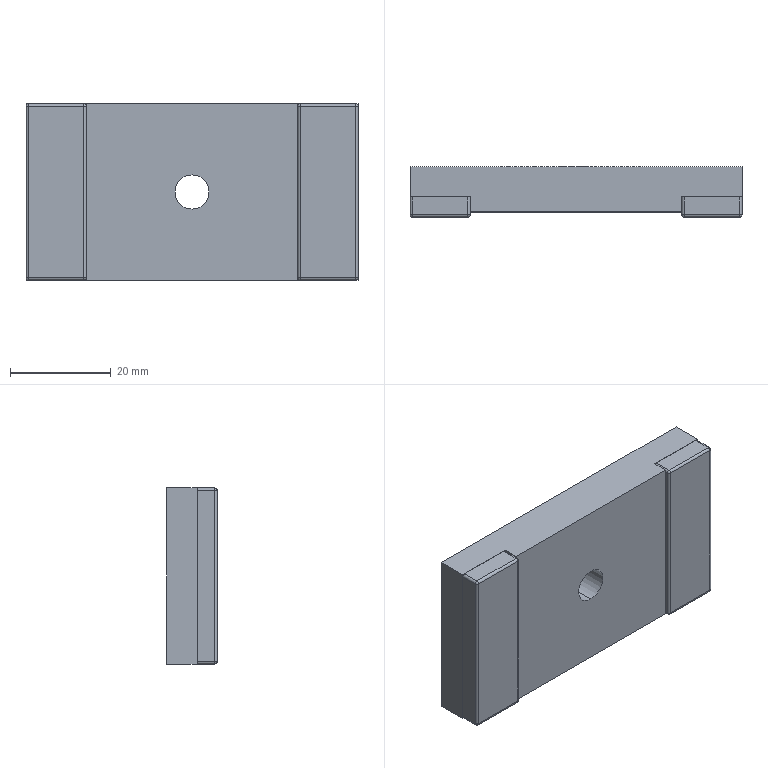Part | SolidWorks | features Fillet 3, Extrusion 1, HoleWzd 1, ICE 1 | 3 solids | 48 faces | box 66 x 10 x 35 mm | volume 21292 mm3 | plane 22 | cylinder 18 | sphere 8 | commonest cylinder face diameters 1 x16 6.8 x2
STEP:
#1=CARTESIAN_POINT('',(-33.,-3.,17.));
#2=VERTEX_POINT('',#1);
#3=CARTESIAN_POINT('',(-33.,-3.,-17.));
#4=VERTEX_POINT('',#3);
#5=CARTESIAN_POINT('',(-33.,-3.,17.5));
#6=DIRECTION('',(0.,0.,-1.));
#7=VECTOR('',#6,1000.);
#8=LINE('',#5,#7);
#9=EDGE_CURVE('',#2,#4,#8,.T.);
#10=ORIENTED_EDGE('',*,*,#9,.T.);
#11=CARTESIAN_POINT('',(-33.,-6.5,-17.));
#12=VERTEX_POINT('',#11);
#13=CARTESIAN_POINT('',(-33.,-7.,-17.));
#14=DIRECTION('',(0.,-1.,0.));
#15=VECTOR('',#14,1000.);
#16=LINE('',#13,#15);
#17=EDGE_CURVE('',#4,#12,#16,.T.);
#18=ORIENTED_EDGE('',*,*,#17,.T.);
#19=CARTESIAN_POINT('',(-33.,-6.5,17.));
#20=VERTEX_POINT('',#19);
#21=CARTESIAN_POINT('',(-33.,-6.5,17.5));
#22=DIRECTION('',(0.,0.,1.));
#23=VECTOR('',#22,1000.);
#24=LINE('',#21,#23);
#25=EDGE_CURVE('',#12,#20,#24,.T.);
#26=ORIENTED_EDGE('',*,*,#25,.T.);
#27=CARTESIAN_POINT('',(-33.,-7.,17.));
#28=DIRECTION('',(0.,1.,0.));
#29=VECTOR('',#28,1000.);
#30=LINE('',#27,#29);
#31=EDGE_CURVE('',#20,#2,#30,.T.);
#32=ORIENTED_EDGE('',*,*,#31,.T.);
#33=EDGE_LOOP('',(#10,#18,#26,#32));
#34=FACE_OUTER_BOUND('',#33,.T.);
#35=CARTESIAN_POINT('',(-33.,-7.,17.5));
#36=DIRECTION('',(1.,0.,0.));
#37=DIRECTION('',(0.,1.,0.));
#38=AXIS2_PLACEMENT_3D('',#35,#36,#37);
#39=PLANE('',#38);
#40=ADVANCED_FACE('',(#34),#39,.F.);
#41=CARTESIAN_POINT('',(-32.5,-3.,-17.5));
#42=VERTEX_POINT('',#41);
#43=CARTESIAN_POINT('',(-21.5,-3.,-17.5));
#44=VERTEX_POINT('',#43);
#45=CARTESIAN_POINT('',(-33.,-3.,-17.5));
#46=DIRECTION('',(1.,0.,0.));
#47=VECTOR('',#46,1000.);
#48=LINE('',#45,#47);
#49=EDGE_CURVE('',#42,#44,#48,.T.);
#50=ORIENTED_EDGE('',*,*,#49,.T.);
#51=CARTESIAN_POINT('',(-21.5,-6.5,-17.5));
#52=VERTEX_POINT('',#51);
#53=CARTESIAN_POINT('',(-21.5,-7.,-17.5));
#54=DIRECTION('',(0.,-1.,0.));
#55=VECTOR('',#54,1000.);
#56=LINE('',#53,#55);
#57=EDGE_CURVE('',#44,#52,#56,.T.);
#58=ORIENTED_EDGE('',*,*,#57,.T.);
#59=CARTESIAN_POINT('',(-32.5,-6.5,-17.5));
#60=VERTEX_POINT('',#59);
#61=CARTESIAN_POINT('',(-33.,-6.5,-17.5));
#62=DIRECTION('',(-1.,0.,0.));
#63=VECTOR('',#62,1000.);
#64=LINE('',#61,#63);
#65=EDGE_CURVE('',#52,#60,#64,.T.);
#66=ORIENTED_EDGE('',*,*,#65,.T.);
#67=CARTESIAN_POINT('',(-32.5,-7.,-17.5));
#68=DIRECTION('',(0.,1.,0.));
#69=VECTOR('',#68,1000.);
#70=LINE('',#67,#69);
#71=EDGE_CURVE('',#60,#42,#70,.T.);
#72=ORIENTED_EDGE('',*,*,#71,.T.);
#73=EDGE_LOOP('',(#50,#58,#66,#72));
#74=FACE_OUTER_BOUND('',#73,.T.);
#75=CARTESIAN_POINT('',(-33.,-7.,-17.5));
#76=DIRECTION('',(0.,0.,1.));
#77=DIRECTION('',(1.,0.,0.));
#78=AXIS2_PLACEMENT_3D('',#75,#76,#77);
#79=PLANE('',#78);
#80=ADVANCED_FACE('',(#74),#79,.F.);
#81=CARTESIAN_POINT('',(-21.,-6.5,17.));
#82=VERTEX_POINT('',#81);
#83=CARTESIAN_POINT('',(-21.,-6.5,-17.));
#84=VERTEX_POINT('',#83);
#85=CARTESIAN_POINT('',(-21.,-6.5,-17.5));
#86=DIRECTION('',(0.,0.,-1.));
#87=VECTOR('',#86,1000.);
#88=LINE('',#85,#87);
#89=EDGE_CURVE('',#82,#84,#88,.T.);
#90=ORIENTED_EDGE('',*,*,#89,.T.);
#91=CARTESIAN_POINT('',(-21.,-3.,-17.));
#92=VERTEX_POINT('',#91);
#93=CARTESIAN_POINT('',(-21.,-7.,-17.));
#94=DIRECTION('',(0.,1.,0.));
#95=VECTOR('',#94,1000.);
#96=LINE('',#93,#95);
#97=EDGE_CURVE('',#84,#92,#96,.T.);
#98=ORIENTED_EDGE('',*,*,#97,.T.);
#99=CARTESIAN_POINT('',(-21.,-3.,17.));
#100=VERTEX_POINT('',#99);
#101=CARTESIAN_POINT('',(-21.,-3.,17.5));
#102=DIRECTION('',(0.,0.,1.));
#103=VECTOR('',#102,1000.);
#104=LINE('',#101,#103);
#105=EDGE_CURVE('',#92,#100,#104,.T.);
#106=ORIENTED_EDGE('',*,*,#105,.T.);
#107=CARTESIAN_POINT('',(-21.,-7.,17.));
#108=DIRECTION('',(0.,-1.,0.));
#109=VECTOR('',#108,1000.);
#110=LINE('',#107,#109);
#111=EDGE_CURVE('',#100,#82,#110,.T.);
#112=ORIENTED_EDGE('',*,*,#111,.T.);
#113=EDGE_LOOP('',(#90,#98,#106,#112));
#114=FACE_OUTER_BOUND('',#113,.T.);
#115=CARTESIAN_POINT('',(-21.,-7.,17.5));
#116=DIRECTION('',(-1.,0.,0.));
#117=DIRECTION('',(0.,-1.,0.));
#118=AXIS2_PLACEMENT_3D('',#115,#116,#117);
#119=PLANE('',#118);
#120=ADVANCED_FACE('',(#114),#119,.F.);
#121=CARTESIAN_POINT('',(-32.5,-6.5,17.5));
#122=VERTEX_POINT('',#121);
#123=CARTESIAN_POINT('',(-21.5,-6.5,17.5));
#124=VERTEX_POINT('',#123);
#125=CARTESIAN_POINT('',(-21.,-6.5,17.5));
#126=DIRECTION('',(1.,0.,0.));
#127=VECTOR('',#126,1000.);
#128=LINE('',#125,#127);
#129=EDGE_CURVE('',#122,#124,#128,.T.);
#130=ORIENTED_EDGE('',*,*,#129,.T.);
#131=CARTESIAN_POINT('',(-21.5,-3.,17.5));
#132=VERTEX_POINT('',#131);
#133=CARTESIAN_POINT('',(-21.5,-7.,17.5));
#134=DIRECTION('',(0.,1.,0.));
#135=VECTOR('',#134,1000.);
#136=LINE('',#133,#135);
#137=EDGE_CURVE('',#124,#132,#136,.T.);
#138=ORIENTED_EDGE('',*,*,#137,.T.);
#139=CARTESIAN_POINT('',(-32.5,-3.,17.5));
#140=VERTEX_POINT('',#139);
#141=CARTESIAN_POINT('',(-33.,-3.,17.5));
#142=DIRECTION('',(-1.,0.,0.));
#143=VECTOR('',#142,1000.);
#144=LINE('',#141,#143);
#145=EDGE_CURVE('',#132,#140,#144,.T.);
#146=ORIENTED_EDGE('',*,*,#145,.T.);
#147=CARTESIAN_POINT('',(-32.5,-7.,17.5));
#148=DIRECTION('',(0.,-1.,0.));
#149=VECTOR('',#148,1000.);
#150=LINE('',#147,#149);
#151=EDGE_CURVE('',#140,#122,#150,.T.);
#152=ORIENTED_EDGE('',*,*,#151,.T.);
#153=EDGE_LOOP('',(#130,#138,#146,#152));
#154=FACE_OUTER_BOUND('',#153,.T.);
#155=CARTESIAN_POINT('',(-33.,-7.,17.5));
#156=DIRECTION('',(0.,0.,-1.));
#157=DIRECTION('',(-1.,0.,0.));
#158=AXIS2_PLACEMENT_3D('',#155,#156,#157);
#159=PLANE('',#158);
#160=ADVANCED_FACE('',(#154),#159,.F.);
#161=CARTESIAN_POINT('',(-21.5,-7.,-17.));
#162=VERTEX_POINT('',#161);
#163=CARTESIAN_POINT('',(-21.5,-7.,17.));
#164=VERTEX_POINT('',#163);
#165=CARTESIAN_POINT('',(-21.5,-7.,17.5));
#166=DIRECTION('',(0.,0.,1.));
#167=VECTOR('',#166,1000.);
#168=LINE('',#165,#167);
#169=EDGE_CURVE('',#162,#164,#168,.T.);
#170=ORIENTED_EDGE('',*,*,#169,.T.);
#171=CARTESIAN_POINT('',(-32.5,-7.,17.));
#172=VERTEX_POINT('',#171);
#173=CARTESIAN_POINT('',(-33.,-7.,17.));
#174=DIRECTION('',(-1.,0.,0.));
#175=VECTOR('',#174,1000.);
#176=LINE('',#173,#175);
#177=EDGE_CURVE('',#164,#172,#176,.T.);
#178=ORIENTED_EDGE('',*,*,#177,.T.);
#179=CARTESIAN_POINT('',(-32.5,-7.,-17.));
#180=VERTEX_POINT('',#179);
#181=CARTESIAN_POINT('',(-32.5,-7.,-17.5));
#182=DIRECTION('',(0.,0.,-1.));
#183=VECTOR('',#182,1000.);
#184=LINE('',#181,#183);
#185=EDGE_CURVE('',#172,#180,#184,.T.);
#186=ORIENTED_EDGE('',*,*,#185,.T.);
#187=CARTESIAN_POINT('',(-21.,-7.,-17.));
#188=DIRECTION('',(1.,0.,0.));
#189=VECTOR('',#188,1000.);
#190=LINE('',#187,#189);
#191=EDGE_CURVE('',#180,#162,#190,.T.);
#192=ORIENTED_EDGE('',*,*,#191,.T.);
#193=EDGE_LOOP('',(#170,#178,#186,#192));
#194=FACE_OUTER_BOUND('',#193,.T.);
#195=CARTESIAN_POINT('',(0.,-7.,0.));
#196=DIRECTION('',(0.,-1.,0.));
#197=DIRECTION('',(1.,0.,0.));
#198=AXIS2_PLACEMENT_3D('',#195,#196,#197);
#199=PLANE('',#198);
#200=ADVANCED_FACE('',(#194),#199,.T.);
#201=ORIENTED_EDGE('',*,*,#105,.F.);
#202=CARTESIAN_POINT('',(-21.5,-3.,-17.));
#203=DIRECTION('',(0.,1.,0.));
#204=DIRECTION('',(1.,0.,0.));
#205=AXIS2_PLACEMENT_3D('',#202,#203,#204);
#206=CIRCLE('',#205,0.5);
#207=EDGE_CURVE('',#92,#44,#206,.T.);
#208=ORIENTED_EDGE('',*,*,#207,.T.);
#209=ORIENTED_EDGE('',*,*,#49,.F.);
#210=CARTESIAN_POINT('',(-32.5,-3.,-17.));
#211=DIRECTION('',(0.,1.,0.));
#212=DIRECTION('',(1.,0.,0.));
#213=AXIS2_PLACEMENT_3D('',#210,#211,#212);
#214=CIRCLE('',#213,0.5);
#215=EDGE_CURVE('',#42,#4,#214,.T.);
#216=ORIENTED_EDGE('',*,*,#215,.T.);
#217=ORIENTED_EDGE('',*,*,#9,.F.);
#218=CARTESIAN_POINT('',(-32.5,-3.,17.));
#219=DIRECTION('',(0.,1.,0.));
#220=DIRECTION('',(1.,0.,0.));
#221=AXIS2_PLACEMENT_3D('',#218,#219,#220);
#222=CIRCLE('',#221,0.5);
#223=EDGE_CURVE('',#2,#140,#222,.T.);
#224=ORIENTED_EDGE('',*,*,#223,.T.);
#225=ORIENTED_EDGE('',*,*,#145,.F.);
#226=CARTESIAN_POINT('',(-21.5,-3.,17.));
#227=DIRECTION('',(0.,1.,0.));
#228=DIRECTION('',(1.,0.,0.));
#229=AXIS2_PLACEMENT_3D('',#226,#227,#228);
#230=CIRCLE('',#229,0.5);
#231=EDGE_CURVE('',#132,#100,#230,.T.);
#232=ORIENTED_EDGE('',*,*,#231,.T.);
#233=EDGE_LOOP('',(#201,#208,#209,#216,#217,#224,#225,#232));
#234=FACE_OUTER_BOUND('',#233,.T.);
#235=CARTESIAN_POINT('',(0.,-3.,0.));
#236=DIRECTION('',(0.,-1.,0.));
#237=DIRECTION('',(1.,0.,0.));
#238=AXIS2_PLACEMENT_3D('',#235,#236,#237);
#239=PLANE('',#238);
#240=ADVANCED_FACE('',(#234),#239,.F.);
#241=ORIENTED_EDGE('',*,*,#65,.F.);
#242=CARTESIAN_POINT('',(-21.5,-6.5,-17.));
#243=DIRECTION('',(-1.,0.,0.));
#244=DIRECTION('',(0.,-1.,0.));
#245=AXIS2_PLACEMENT_3D('',#242,#243,#244);
#246=CIRCLE('',#245,0.5);
#247=EDGE_CURVE('',#52,#162,#246,.T.);
#248=ORIENTED_EDGE('',*,*,#247,.T.);
#249=ORIENTED_EDGE('',*,*,#191,.F.);
#250=CARTESIAN_POINT('',(-32.5,-6.5,-17.));
#251=DIRECTION('',(1.,0.,0.));
#252=DIRECTION('',(0.,-1.,0.));
#253=AXIS2_PLACEMENT_3D('',#250,#251,#252);
#254=CIRCLE('',#253,0.5);
#255=EDGE_CURVE('',#180,#60,#254,.T.);
#256=ORIENTED_EDGE('',*,*,#255,.T.);
#257=EDGE_LOOP('',(#241,#248,#249,#256));
#258=FACE_OUTER_BOUND('',#257,.T.);
#259=CARTESIAN_POINT('',(0.,-6.5,-17.));
#260=DIRECTION('',(-1.,0.,0.));
#261=DIRECTION('',(0.,-1.,0.));
#262=AXIS2_PLACEMENT_3D('',#259,#260,#261);
#263=CYLINDRICAL_SURFACE('',#262,0.5);
#264=ADVANCED_FACE('',(#258),#263,.T.);
#265=ORIENTED_EDGE('',*,*,#169,.F.);
#266=CARTESIAN_POINT('',(-21.5,-6.5,-17.));
#267=DIRECTION('',(0.,0.,1.));
#268=DIRECTION('',(-1.,0.,0.));
#269=AXIS2_PLACEMENT_3D('',#266,#267,#268);
#270=CIRCLE('',#269,0.5);
#271=EDGE_CURVE('',#162,#84,#270,.T.);
#272=ORIENTED_EDGE('',*,*,#271,.T.);
#273=ORIENTED_EDGE('',*,*,#89,.F.);
#274=CARTESIAN_POINT('',(-21.5,-6.5,17.));
#275=DIRECTION('',(0.,0.,-1.));
#276=DIRECTION('',(-1.,0.,0.));
#277=AXIS2_PLACEMENT_3D('',#274,#275,#276);
#278=CIRCLE('',#277,0.5);
#279=EDGE_CURVE('',#82,#164,#278,.T.);
#280=ORIENTED_EDGE('',*,*,#279,.T.);
#281=EDGE_LOOP('',(#265,#272,#273,#280));
#282=FACE_OUTER_BOUND('',#281,.T.);
#283=CARTESIAN_POINT('',(-21.5,-6.5,0.));
#284=DIRECTION('',(0.,0.,-1.));
#285=DIRECTION('',(-1.,0.,0.));
#286=AXIS2_PLACEMENT_3D('',#283,#284,#285);
#287=CYLINDRICAL_SURFACE('',#286,0.5);
#288=ADVANCED_FACE('',(#282),#287,.T.);
#289=ORIENTED_EDGE('',*,*,#25,.F.);
#290=CARTESIAN_POINT('',(-32.5,-6.5,-17.));
#291=DIRECTION('',(0.,0.,1.));
#292=DIRECTION('',(1.,0.,0.));
#293=AXIS2_PLACEMENT_3D('',#290,#291,#292);
#294=CIRCLE('',#293,0.5);
#295=EDGE_CURVE('',#12,#180,#294,.T.);
#296=ORIENTED_EDGE('',*,*,#295,.T.);
#297=ORIENTED_EDGE('',*,*,#185,.F.);
#298=CARTESIAN_POINT('',(-32.5,-6.5,17.));
#299=DIRECTION('',(0.,0.,-1.));
#300=DIRECTION('',(1.,0.,0.));
#301=AXIS2_PLACEMENT_3D('',#298,#299,#300);
#302=CIRCLE('',#301,0.5);
#303=EDGE_CURVE('',#172,#20,#302,.T.);
#304=ORIENTED_EDGE('',*,*,#303,.T.);
#305=EDGE_LOOP('',(#289,#296,#297,#304));
#306=FACE_OUTER_BOUND('',#305,.T.);
#307=CARTESIAN_POINT('',(-32.5,-6.5,0.));
#308=DIRECTION('',(0.,0.,1.));
#309=DIRECTION('',(1.,0.,0.));
#310=AXIS2_PLACEMENT_3D('',#307,#308,#309);
#311=CYLINDRICAL_SURFACE('',#310,0.5);
#312=ADVANCED_FACE('',(#306),#311,.T.);
#313=ORIENTED_EDGE('',*,*,#177,.F.);
#314=CARTESIAN_POINT('',(-21.5,-6.5,17.));
#315=DIRECTION('',(-1.,0.,0.));
#316=DIRECTION('',(0.,1.,0.));
#317=AXIS2_PLACEMENT_3D('',#314,#315,#316);
#318=CIRCLE('',#317,0.5);
#319=EDGE_CURVE('',#164,#124,#318,.T.);
#320=ORIENTED_EDGE('',*,*,#319,.T.);
#321=ORIENTED_EDGE('',*,*,#129,.F.);
#322=CARTESIAN_POINT('',(-32.5,-6.5,17.));
#323=DIRECTION('',(1.,0.,0.));
#324=DIRECTION('',(0.,1.,0.));
#325=AXIS2_PLACEMENT_3D('',#322,#323,#324);
#326=CIRCLE('',#325,0.5);
#327=EDGE_CURVE('',#122,#172,#326,.T.);
#328=ORIENTED_EDGE('',*,*,#327,.T.);
#329=EDGE_LOOP('',(#313,#320,#321,#328));
#330=FACE_OUTER_BOUND('',#329,.T.);
#331=CARTESIAN_POINT('',(0.,-6.5,17.));
#332=DIRECTION('',(1.,0.,0.));
#333=DIRECTION('',(0.,1.,0.));
#334=AXIS2_PLACEMENT_3D('',#331,#332,#333);
#335=CYLINDRICAL_SURFACE('',#334,0.5);
#336=ADVANCED_FACE('',(#330),#335,.T.);
#337=ORIENTED_EDGE('',*,*,#207,.F.);
#338=ORIENTED_EDGE('',*,*,#97,.F.);
#339=CARTESIAN_POINT('',(-21.5,-6.5,-17.));
#340=DIRECTION('',(0.,-1.,0.));
#341=DIRECTION('',(1.,0.,0.));
#342=AXIS2_PLACEMENT_3D('',#339,#340,#341);
#343=CIRCLE('',#342,0.5);
#344=EDGE_CURVE('',#52,#84,#343,.T.);
#345=ORIENTED_EDGE('',*,*,#344,.F.);
#346=ORIENTED_EDGE('',*,*,#57,.F.);
#347=EDGE_LOOP('',(#337,#338,#345,#346));
#348=FACE_OUTER_BOUND('',#347,.T.);
#349=CARTESIAN_POINT('',(-21.5,-7.,-17.));
#350=DIRECTION('',(0.,1.,0.));
#351=DIRECTION('',(-1.,0.,0.));
#352=AXIS2_PLACEMENT_3D('',#349,#350,#351);
#353=CYLINDRICAL_SURFACE('',#352,0.5);
#354=ADVANCED_FACE('',(#348),#353,.T.);
#355=ORIENTED_EDGE('',*,*,#271,.F.);
#356=ORIENTED_EDGE('',*,*,#247,.F.);
#357=ORIENTED_EDGE('',*,*,#344,.T.);
#358=EDGE_LOOP('',(#355,#356,#357));
#359=FACE_OUTER_BOUND('',#358,.T.);
#360=CARTESIAN_POINT('',(-21.5,-6.5,-17.));
#361=DIRECTION('',(0.,1.,0.));
#362=DIRECTION('',(1.,0.,0.));
#363=AXIS2_PLACEMENT_3D('',#360,#361,#362);
#364=SPHERICAL_SURFACE('',#363,0.5);
#365=ADVANCED_FACE('',(#359),#364,.T.);
#366=ORIENTED_EDGE('',*,*,#215,.F.);
#367=ORIENTED_EDGE('',*,*,#71,.F.);
#368=CARTESIAN_POINT('',(-32.5,-6.5,-17.));
#369=DIRECTION('',(0.,-1.,0.));
#370=DIRECTION('',(1.,0.,0.));
#371=AXIS2_PLACEMENT_3D('',#368,#369,#370);
#372=CIRCLE('',#371,0.5);
#373=EDGE_CURVE('',#12,#60,#372,.T.);
#374=ORIENTED_EDGE('',*,*,#373,.F.);
#375=ORIENTED_EDGE('',*,*,#17,.F.);
#376=EDGE_LOOP('',(#366,#367,#374,#375));
#377=FACE_OUTER_BOUND('',#376,.T.);
#378=CARTESIAN_POINT('',(-32.5,-7.,-17.));
#379=DIRECTION('',(0.,1.,0.));
#380=DIRECTION('',(-1.,0.,0.));
#381=AXIS2_PLACEMENT_3D('',#378,#379,#380);
#382=CYLINDRICAL_SURFACE('',#381,0.5);
#383=ADVANCED_FACE('',(#377),#382,.T.);
#384=ORIENTED_EDGE('',*,*,#373,.T.);
#385=ORIENTED_EDGE('',*,*,#255,.F.);
#386=ORIENTED_EDGE('',*,*,#295,.F.);
#387=EDGE_LOOP('',(#384,#385,#386));
#388=FACE_OUTER_BOUND('',#387,.T.);
#389=CARTESIAN_POINT('',(-32.5,-6.5,-17.));
#390=DIRECTION('',(0.,1.,0.));
#391=DIRECTION('',(1.,0.,0.));
#392=AXIS2_PLACEMENT_3D('',#389,#390,#391);
#393=SPHERICAL_SURFACE('',#392,0.5);
#394=ADVANCED_FACE('',(#388),#393,.T.);
#395=ORIENTED_EDGE('',*,*,#231,.F.);
#396=ORIENTED_EDGE('',*,*,#137,.F.);
#397=CARTESIAN_POINT('',(-21.5,-6.5,17.));
#398=DIRECTION('',(0.,-1.,0.));
#399=DIRECTION('',(1.,0.,0.));
#400=AXIS2_PLACEMENT_3D('',#397,#398,#399);
#401=CIRCLE('',#400,0.5);
#402=EDGE_CURVE('',#82,#124,#401,.T.);
#403=ORIENTED_EDGE('',*,*,#402,.F.);
#404=ORIENTED_EDGE('',*,*,#111,.F.);
#405=EDGE_LOOP('',(#395,#396,#403,#404));
#406=FACE_OUTER_BOUND('',#405,.T.);
#407=CARTESIAN_POINT('',(-21.5,-7.,17.));
#408=DIRECTION('',(0.,1.,0.));
#409=DIRECTION('',(-1.,0.,0.));
#410=AXIS2_PLACEMENT_3D('',#407,#408,#409);
#411=CYLINDRICAL_SURFACE('',#410,0.5);
#412=ADVANCED_FACE('',(#406),#411,.T.);
#413=ORIENTED_EDGE('',*,*,#319,.F.);
#414=ORIENTED_EDGE('',*,*,#279,.F.);
#415=ORIENTED_EDGE('',*,*,#402,.T.);
#416=EDGE_LOOP('',(#413,#414,#415));
#417=FACE_OUTER_BOUND('',#416,.T.);
#418=CARTESIAN_POINT('',(-21.5,-6.5,17.));
#419=DIRECTION('',(0.,1.,0.));
#420=DIRECTION('',(1.,0.,0.));
#421=AXIS2_PLACEMENT_3D('',#418,#419,#420);
#422=SPHERICAL_SURFACE('',#421,0.5);
#423=ADVANCED_FACE('',(#417),#422,.T.);
#424=ORIENTED_EDGE('',*,*,#223,.F.);
#425=ORIENTED_EDGE('',*,*,#31,.F.);
#426=CARTESIAN_POINT('',(-32.5,-6.5,17.));
#427=DIRECTION('',(0.,-1.,0.));
#428=DIRECTION('',(1.,0.,0.));
#429=AXIS2_PLACEMENT_3D('',#426,#427,#428);
#430=CIRCLE('',#429,0.5);
#431=EDGE_CURVE('',#122,#20,#430,.T.);
#432=ORIENTED_EDGE('',*,*,#431,.F.);
#433=ORIENTED_EDGE('',*,*,#151,.F.);
#434=EDGE_LOOP('',(#424,#425,#432,#433));
#435=FACE_OUTER_BOUND('',#434,.T.);
#436=CARTESIAN_POINT('',(-32.5,-7.,17.));
#437=DIRECTION('',(0.,1.,0.));
#438=DIRECTION('',(-1.,0.,0.));
#439=AXIS2_PLACEMENT_3D('',#436,#437,#438);
#440=CYLINDRICAL_SURFACE('',#439,0.5);
#441=ADVANCED_FACE('',(#435),#440,.T.);
#442=ORIENTED_EDGE('',*,*,#431,.T.);
#443=ORIENTED_EDGE('',*,*,#303,.F.);
#444=ORIENTED_EDGE('',*,*,#327,.F.);
#445=EDGE_LOOP('',(#442,#443,#444));
#446=FACE_OUTER_BOUND('',#445,.T.);
#447=CARTESIAN_POINT('',(-32.5,-6.5,17.));
#448=DIRECTION('',(0.,1.,0.));
#449=DIRECTION('',(1.,0.,0.));
#450=AXIS2_PLACEMENT_3D('',#447,#448,#449);
#451=SPHERICAL_SURFACE('',#450,0.5);
#452=ADVANCED_FACE('',(#446),#451,.T.);
#453=CLOSED_SHELL('',(#40,#80,#120,#160,#200,#240,#264,#288,#312,#336,#354,#365,#383,#394,#412,#423,#441,#452));
#454=MANIFOLD_SOLID_BREP('',#453);
#455=CARTESIAN_POINT('',(21.,-6.5,-17.));
#456=VERTEX_POINT('',#455);
#457=CARTESIAN_POINT('',(21.,-6.5,17.));
#458=VERTEX_POINT('',#457);
#459=CARTESIAN_POINT('',(21.,-6.5,17.5));
#460=DIRECTION('',(0.,0.,1.));
#461=VECTOR('',#460,1000.);
#462=LINE('',#459,#461);
#463=EDGE_CURVE('',#456,#458,#462,.T.);
#464=ORIENTED_EDGE('',*,*,#463,.T.);
#465=CARTESIAN_POINT('',(21.,-3.,17.));
#466=VERTEX_POINT('',#465);
#467=CARTESIAN_POINT('',(21.,-7.,17.));
#468=DIRECTION('',(0.,1.,0.));
#469=VECTOR('',#468,1000.);
#470=LINE('',#467,#469);
#471=EDGE_CURVE('',#458,#466,#470,.T.);
#472=ORIENTED_EDGE('',*,*,#471,.T.);
#473=CARTESIAN_POINT('',(21.,-3.,-17.));
#474=VERTEX_POINT('',#473);
#475=CARTESIAN_POINT('',(21.,-3.,17.5));
#476=DIRECTION('',(0.,0.,-1.));
#477=VECTOR('',#476,1000.);
#478=LINE('',#475,#477);
#479=EDGE_CURVE('',#466,#474,#478,.T.);
#480=ORIENTED_EDGE('',*,*,#479,.T.);
#481=CARTESIAN_POINT('',(21.,-7.,-17.));
#482=DIRECTION('',(0.,-1.,0.));
#483=VECTOR('',#482,1000.);
#484=LINE('',#481,#483);
#485=EDGE_CURVE('',#474,#456,#484,.T.);
#486=ORIENTED_EDGE('',*,*,#485,.T.);
#487=EDGE_LOOP('',(#464,#472,#480,#486));
#488=FACE_OUTER_BOUND('',#487,.T.);
#489=CARTESIAN_POINT('',(21.,-7.,17.5));
#490=DIRECTION('',(1.,0.,0.));
#491=DIRECTION('',(0.,1.,0.));
#492=AXIS2_PLACEMENT_3D('',#489,#490,#491);
#493=PLANE('',#492);
#494=ADVANCED_FACE('',(#488),#493,.F.);
#495=CARTESIAN_POINT('',(21.5,-3.,-17.5));
#496=VERTEX_POINT('',#495);
#497=CARTESIAN_POINT('',(32.5,-3.,-17.5));
#498=VERTEX_POINT('',#497);
#499=CARTESIAN_POINT('',(21.,-3.,-17.5));
#500=DIRECTION('',(1.,0.,0.));
#501=VECTOR('',#500,1000.);
#502=LINE('',#499,#501);
#503=EDGE_CURVE('',#496,#498,#502,.T.);
#504=ORIENTED_EDGE('',*,*,#503,.T.);
#505=CARTESIAN_POINT('',(32.5,-6.5,-17.5));
#506=VERTEX_POINT('',#505);
#507=CARTESIAN_POINT('',(32.5,-7.,-17.5));
#508=DIRECTION('',(0.,-1.,0.));
#509=VECTOR('',#508,1000.);
#510=LINE('',#507,#509);
#511=EDGE_CURVE('',#498,#506,#510,.T.);
#512=ORIENTED_EDGE('',*,*,#511,.T.);
#513=CARTESIAN_POINT('',(21.5,-6.5,-17.5));
#514=VERTEX_POINT('',#513);
#515=CARTESIAN_POINT('',(21.,-6.5,-17.5));
#516=DIRECTION('',(-1.,0.,0.));
#517=VECTOR('',#516,1000.);
#518=LINE('',#515,#517);
#519=EDGE_CURVE('',#506,#514,#518,.T.);
#520=ORIENTED_EDGE('',*,*,#519,.T.);
#521=CARTESIAN_POINT('',(21.5,-7.,-17.5));
#522=DIRECTION('',(0.,1.,0.));
#523=VECTOR('',#522,1000.);
#524=LINE('',#521,#523);
#525=EDGE_CURVE('',#514,#496,#524,.T.);
#526=ORIENTED_EDGE('',*,*,#525,.T.);
#527=EDGE_LOOP('',(#504,#512,#520,#526));
#528=FACE_OUTER_BOUND('',#527,.T.);
#529=CARTESIAN_POINT('',(21.,-7.,-17.5));
#530=DIRECTION('',(0.,0.,1.));
#531=DIRECTION('',(1.,0.,0.));
#532=AXIS2_PLACEMENT_3D('',#529,#530,#531);
#533=PLANE('',#532);
#534=ADVANCED_FACE('',(#528),#533,.F.);
#535=CARTESIAN_POINT('',(33.,-6.5,17.));
#536=VERTEX_POINT('',#535);
#537=CARTESIAN_POINT('',(33.,-6.5,-17.));
#538=VERTEX_POINT('',#537);
#539=CARTESIAN_POINT('',(33.,-6.5,-17.5));
#540=DIRECTION('',(0.,0.,-1.));
#541=VECTOR('',#540,1000.);
#542=LINE('',#539,#541);
#543=EDGE_CURVE('',#536,#538,#542,.T.);
#544=ORIENTED_EDGE('',*,*,#543,.T.);
#545=CARTESIAN_POINT('',(33.,-3.,-17.));
#546=VERTEX_POINT('',#545);
#547=CARTESIAN_POINT('',(33.,-7.,-17.));
#548=DIRECTION('',(0.,1.,0.));
#549=VECTOR('',#548,1000.);
#550=LINE('',#547,#549);
#551=EDGE_CURVE('',#538,#546,#550,.T.);
#552=ORIENTED_EDGE('',*,*,#551,.T.);
#553=CARTESIAN_POINT('',(33.,-3.,17.));
#554=VERTEX_POINT('',#553);
#555=CARTESIAN_POINT('',(33.,-3.,17.5));
#556=DIRECTION('',(0.,0.,1.));
#557=VECTOR('',#556,1000.);
#558=LINE('',#555,#557);
#559=EDGE_CURVE('',#546,#554,#558,.T.);
#560=ORIENTED_EDGE('',*,*,#559,.T.);
#561=CARTESIAN_POINT('',(33.,-7.,17.));
#562=DIRECTION('',(0.,-1.,0.));
#563=VECTOR('',#562,1000.);
#564=LINE('',#561,#563);
#565=EDGE_CURVE('',#554,#536,#564,.T.);
#566=ORIENTED_EDGE('',*,*,#565,.T.);
#567=EDGE_LOOP('',(#544,#552,#560,#566));
#568=FACE_OUTER_BOUND('',#567,.T.);
#569=CARTESIAN_POINT('',(33.,-7.,17.5));
#570=DIRECTION('',(-1.,0.,0.));
#571=DIRECTION('',(0.,-1.,0.));
#572=AXIS2_PLACEMENT_3D('',#569,#570,#571);
#573=PLANE('',#572);
#574=ADVANCED_FACE('',(#568),#573,.F.);
#575=CARTESIAN_POINT('',(32.5,-3.,17.5));
#576=VERTEX_POINT('',#575);
#577=CARTESIAN_POINT('',(21.5,-3.,17.5));
#578=VERTEX_POINT('',#577);
#579=CARTESIAN_POINT('',(21.,-3.,17.5));
#580=DIRECTION('',(-1.,0.,0.));
#581=VECTOR('',#580,1000.);
#582=LINE('',#579,#581);
#583=EDGE_CURVE('',#576,#578,#582,.T.);
#584=ORIENTED_EDGE('',*,*,#583,.T.);
#585=CARTESIAN_POINT('',(21.5,-6.5,17.5));
#586=VERTEX_POINT('',#585);
#587=CARTESIAN_POINT('',(21.5,-7.,17.5));
#588=DIRECTION('',(0.,-1.,0.));
#589=VECTOR('',#588,1000.);
#590=LINE('',#587,#589);
#591=EDGE_CURVE('',#578,#586,#590,.T.);
#592=ORIENTED_EDGE('',*,*,#591,.T.);
#593=CARTESIAN_POINT('',(32.5,-6.5,17.5));
#594=VERTEX_POINT('',#593);
#595=CARTESIAN_POINT('',(33.,-6.5,17.5));
#596=DIRECTION('',(1.,0.,0.));
#597=VECTOR('',#596,1000.);
#598=LINE('',#595,#597);
#599=EDGE_CURVE('',#586,#594,#598,.T.);
#600=ORIENTED_EDGE('',*,*,#599,.T.);
#601=CARTESIAN_POINT('',(32.5,-7.,17.5));
#602=DIRECTION('',(0.,1.,0.));
#603=VECTOR('',#602,1000.);
#604=LINE('',#601,#603);
#605=EDGE_CURVE('',#594,#576,#604,.T.);
#606=ORIENTED_EDGE('',*,*,#605,.T.);
#607=EDGE_LOOP('',(#584,#592,#600,#606));
#608=FACE_OUTER_BOUND('',#607,.T.);
#609=CARTESIAN_POINT('',(21.,-7.,17.5));
#610=DIRECTION('',(0.,0.,-1.));
#611=DIRECTION('',(-1.,0.,0.));
#612=AXIS2_PLACEMENT_3D('',#609,#610,#611);
#613=PLANE('',#612);
#614=ADVANCED_FACE('',(#608),#613,.F.);
#615=CARTESIAN_POINT('',(32.5,-7.,-17.));
#616=VERTEX_POINT('',#615);
#617=CARTESIAN_POINT('',(32.5,-7.,17.));
#618=VERTEX_POINT('',#617);
#619=CARTESIAN_POINT('',(32.5,-7.,17.5));
#620=DIRECTION('',(0.,0.,1.));
#621=VECTOR('',#620,1000.);
#622=LINE('',#619,#621);
#623=EDGE_CURVE('',#616,#618,#622,.T.);
#624=ORIENTED_EDGE('',*,*,#623,.T.);
#625=CARTESIAN_POINT('',(21.5,-7.,17.));
#626=VERTEX_POINT('',#625);
#627=CARTESIAN_POINT('',(21.,-7.,17.));
#628=DIRECTION('',(-1.,0.,0.));
#629=VECTOR('',#628,1000.);
#630=LINE('',#627,#629);
#631=EDGE_CURVE('',#618,#626,#630,.T.);
#632=ORIENTED_EDGE('',*,*,#631,.T.);
#633=CARTESIAN_POINT('',(21.5,-7.,-17.));
#634=VERTEX_POINT('',#633);
#635=CARTESIAN_POINT('',(21.5,-7.,-17.5));
#636=DIRECTION('',(0.,0.,-1.));
#637=VECTOR('',#636,1000.);
#638=LINE('',#635,#637);
#639=EDGE_CURVE('',#626,#634,#638,.T.);
#640=ORIENTED_EDGE('',*,*,#639,.T.);
#641=CARTESIAN_POINT('',(33.,-7.,-17.));
#642=DIRECTION('',(1.,0.,0.));
#643=VECTOR('',#642,1000.);
#644=LINE('',#641,#643);
#645=EDGE_CURVE('',#634,#616,#644,.T.);
#646=ORIENTED_EDGE('',*,*,#645,.T.);
#647=EDGE_LOOP('',(#624,#632,#640,#646));
#648=FACE_OUTER_BOUND('',#647,.T.);
#649=CARTESIAN_POINT('',(0.,-7.,0.));
#650=DIRECTION('',(0.,-1.,0.));
#651=DIRECTION('',(1.,0.,0.));
#652=AXIS2_PLACEMENT_3D('',#649,#650,#651);
#653=PLANE('',#652);
#654=ADVANCED_FACE('',(#648),#653,.T.);
#655=ORIENTED_EDGE('',*,*,#559,.F.);
#656=CARTESIAN_POINT('',(32.5,-3.,-17.));
#657=DIRECTION('',(0.,1.,0.));
#658=DIRECTION('',(1.,0.,0.));
#659=AXIS2_PLACEMENT_3D('',#656,#657,#658);
#660=CIRCLE('',#659,0.5);
#661=EDGE_CURVE('',#546,#498,#660,.T.);
#662=ORIENTED_EDGE('',*,*,#661,.T.);
#663=ORIENTED_EDGE('',*,*,#503,.F.);
#664=CARTESIAN_POINT('',(21.5,-3.,-17.));
#665=DIRECTION('',(0.,1.,0.));
#666=DIRECTION('',(1.,0.,0.));
#667=AXIS2_PLACEMENT_3D('',#664,#665,#666);
#668=CIRCLE('',#667,0.5);
#669=EDGE_CURVE('',#496,#474,#668,.T.);
#670=ORIENTED_EDGE('',*,*,#669,.T.);
#671=ORIENTED_EDGE('',*,*,#479,.F.);
#672=CARTESIAN_POINT('',(21.5,-3.,17.));
#673=DIRECTION('',(0.,1.,0.));
#674=DIRECTION('',(1.,0.,0.));
#675=AXIS2_PLACEMENT_3D('',#672,#673,#674);
#676=CIRCLE('',#675,0.5);
#677=EDGE_CURVE('',#466,#578,#676,.T.);
#678=ORIENTED_EDGE('',*,*,#677,.T.);
#679=ORIENTED_EDGE('',*,*,#583,.F.);
#680=CARTESIAN_POINT('',(32.5,-3.,17.));
#681=DIRECTION('',(0.,1.,0.));
#682=DIRECTION('',(1.,0.,0.));
#683=AXIS2_PLACEMENT_3D('',#680,#681,#682);
#684=CIRCLE('',#683,0.5);
#685=EDGE_CURVE('',#576,#554,#684,.T.);
#686=ORIENTED_EDGE('',*,*,#685,.T.);
#687=EDGE_LOOP('',(#655,#662,#663,#670,#671,#678,#679,#686));
#688=FACE_OUTER_BOUND('',#687,.T.);
#689=CARTESIAN_POINT('',(0.,-3.,0.));
#690=DIRECTION('',(0.,-1.,0.));
#691=DIRECTION('',(1.,0.,0.));
#692=AXIS2_PLACEMENT_3D('',#689,#690,#691);
#693=PLANE('',#692);
#694=ADVANCED_FACE('',(#688),#693,.F.);
#695=ORIENTED_EDGE('',*,*,#661,.F.);
#696=ORIENTED_EDGE('',*,*,#551,.F.);
#697=CARTESIAN_POINT('',(32.5,-6.5,-17.));
#698=DIRECTION('',(0.,-1.,0.));
#699=DIRECTION('',(1.,0.,0.));
#700=AXIS2_PLACEMENT_3D('',#697,#698,#699);
#701=CIRCLE('',#700,0.5);
#702=EDGE_CURVE('',#506,#538,#701,.T.);
#703=ORIENTED_EDGE('',*,*,#702,.F.);
#704=ORIENTED_EDGE('',*,*,#511,.F.);
#705=EDGE_LOOP('',(#695,#696,#703,#704));
#706=FACE_OUTER_BOUND('',#705,.T.);
#707=CARTESIAN_POINT('',(32.5,-7.,-17.));
#708=DIRECTION('',(0.,1.,0.));
#709=DIRECTION('',(-1.,0.,0.));
#710=AXIS2_PLACEMENT_3D('',#707,#708,#709);
#711=CYLINDRICAL_SURFACE('',#710,0.5);
#712=ADVANCED_FACE('',(#706),#711,.T.);
#713=CARTESIAN_POINT('',(21.5,-6.5,-17.));
#714=DIRECTION('',(-1.,0.,0.));
#715=DIRECTION('',(0.,0.,1.));
#716=AXIS2_PLACEMENT_3D('',#713,#714,#715);
#717=CIRCLE('',#716,0.5);
#718=EDGE_CURVE('',#514,#634,#717,.T.);
#719=ORIENTED_EDGE('',*,*,#718,.F.);
#720=ORIENTED_EDGE('',*,*,#519,.F.);
#721=CARTESIAN_POINT('',(32.5,-6.5,-17.));
#722=DIRECTION('',(1.,0.,0.));
#723=DIRECTION('',(0.,0.,-1.));
#724=AXIS2_PLACEMENT_3D('',#721,#722,#723);
#725=CIRCLE('',#724,0.5);
#726=EDGE_CURVE('',#616,#506,#725,.T.);
#727=ORIENTED_EDGE('',*,*,#726,.F.);
#728=ORIENTED_EDGE('',*,*,#645,.F.);
#729=EDGE_LOOP('',(#719,#720,#727,#728));
#730=FACE_OUTER_BOUND('',#729,.T.);
#731=CARTESIAN_POINT('',(0.,-6.5,-17.));
#732=DIRECTION('',(-1.,0.,0.));
#733=DIRECTION('',(0.,-1.,0.));
#734=AXIS2_PLACEMENT_3D('',#731,#732,#733);
#735=CYLINDRICAL_SURFACE('',#734,0.5);
#736=ADVANCED_FACE('',(#730),#735,.T.);
#737=ORIENTED_EDGE('',*,*,#669,.F.);
#738=ORIENTED_EDGE('',*,*,#525,.F.);
#739=CARTESIAN_POINT('',(21.5,-6.5,-17.));
#740=DIRECTION('',(0.,-1.,0.));
#741=DIRECTION('',(1.,0.,0.));
#742=AXIS2_PLACEMENT_3D('',#739,#740,#741);
#743=CIRCLE('',#742,0.5);
#744=EDGE_CURVE('',#456,#514,#743,.T.);
#745=ORIENTED_EDGE('',*,*,#744,.F.);
#746=ORIENTED_EDGE('',*,*,#485,.F.);
#747=EDGE_LOOP('',(#737,#738,#745,#746));
#748=FACE_OUTER_BOUND('',#747,.T.);
#749=CARTESIAN_POINT('',(21.5,-7.,-17.));
#750=DIRECTION('',(0.,1.,0.));
#751=DIRECTION('',(-1.,0.,0.));
#752=AXIS2_PLACEMENT_3D('',#749,#750,#751);
#753=CYLINDRICAL_SURFACE('',#752,0.5);
#754=ADVANCED_FACE('',(#748),#753,.T.);
#755=ORIENTED_EDGE('',*,*,#726,.T.);
#756=ORIENTED_EDGE('',*,*,#702,.T.);
#757=CARTESIAN_POINT('',(32.5,-6.5,-17.));
#758=DIRECTION('',(0.,0.,1.));
#759=DIRECTION('',(-1.,0.,0.));
#760=AXIS2_PLACEMENT_3D('',#757,#758,#759);
#761=CIRCLE('',#760,0.5);
#762=EDGE_CURVE('',#616,#538,#761,.T.);
#763=ORIENTED_EDGE('',*,*,#762,.F.);
#764=EDGE_LOOP('',(#755,#756,#763));
#765=FACE_OUTER_BOUND('',#764,.T.);
#766=CARTESIAN_POINT('',(32.5,-6.5,-17.));
#767=DIRECTION('',(0.,1.,0.));
#768=DIRECTION('',(-1.,0.,0.));
#769=AXIS2_PLACEMENT_3D('',#766,#767,#768);
#770=SPHERICAL_SURFACE('',#769,0.5);
#771=ADVANCED_FACE('',(#765),#770,.T.);
#772=ORIENTED_EDGE('',*,*,#744,.T.);
#773=ORIENTED_EDGE('',*,*,#718,.T.);
#774=CARTESIAN_POINT('',(21.5,-6.5,-17.));
#775=DIRECTION('',(0.,0.,1.));
#776=DIRECTION('',(-1.,0.,0.));
#777=AXIS2_PLACEMENT_3D('',#774,#775,#776);
#778=CIRCLE('',#777,0.5);
#779=EDGE_CURVE('',#456,#634,#778,.T.);
#780=ORIENTED_EDGE('',*,*,#779,.F.);
#781=EDGE_LOOP('',(#772,#773,#780));
#782=FACE_OUTER_BOUND('',#781,.T.);
#783=CARTESIAN_POINT('',(21.5,-6.5,-17.));
#784=DIRECTION('',(0.,1.,0.));
#785=DIRECTION('',(-1.,0.,0.));
#786=AXIS2_PLACEMENT_3D('',#783,#784,#785);
#787=SPHERICAL_SURFACE('',#786,0.5);
#788=ADVANCED_FACE('',(#782),#787,.T.);
#789=ORIENTED_EDGE('',*,*,#685,.F.);
#790=ORIENTED_EDGE('',*,*,#605,.F.);
#791=CARTESIAN_POINT('',(32.5,-6.5,17.));
#792=DIRECTION('',(0.,-1.,0.));
#793=DIRECTION('',(1.,0.,0.));
#794=AXIS2_PLACEMENT_3D('',#791,#792,#793);
#795=CIRCLE('',#794,0.5);
#796=EDGE_CURVE('',#536,#594,#795,.T.);
#797=ORIENTED_EDGE('',*,*,#796,.F.);
#798=ORIENTED_EDGE('',*,*,#565,.F.);
#799=EDGE_LOOP('',(#789,#790,#797,#798));
#800=FACE_OUTER_BOUND('',#799,.T.);
#801=CARTESIAN_POINT('',(32.5,-7.,17.));
#802=DIRECTION('',(0.,1.,0.));
#803=DIRECTION('',(-1.,0.,0.));
#804=AXIS2_PLACEMENT_3D('',#801,#802,#803);
#805=CYLINDRICAL_SURFACE('',#804,0.5);
#806=ADVANCED_FACE('',(#800),#805,.T.);
#807=ORIENTED_EDGE('',*,*,#762,.T.);
#808=ORIENTED_EDGE('',*,*,#543,.F.);
#809=CARTESIAN_POINT('',(32.5,-6.5,17.));
#810=DIRECTION('',(0.,0.,1.));
#811=DIRECTION('',(1.,0.,0.));
#812=AXIS2_PLACEMENT_3D('',#809,#810,#811);
#813=CIRCLE('',#812,0.5);
#814=EDGE_CURVE('',#618,#536,#813,.T.);
#815=ORIENTED_EDGE('',*,*,#814,.F.);
#816=ORIENTED_EDGE('',*,*,#623,.F.);
#817=EDGE_LOOP('',(#807,#808,#815,#816));
#818=FACE_OUTER_BOUND('',#817,.T.);
#819=CARTESIAN_POINT('',(32.5,-6.5,0.));
#820=DIRECTION('',(0.,0.,-1.));
#821=DIRECTION('',(-1.,0.,0.));
#822=AXIS2_PLACEMENT_3D('',#819,#820,#821);
#823=CYLINDRICAL_SURFACE('',#822,0.5);
#824=ADVANCED_FACE('',(#818),#823,.T.);
#825=ORIENTED_EDGE('',*,*,#779,.T.);
#826=ORIENTED_EDGE('',*,*,#639,.F.);
#827=CARTESIAN_POINT('',(21.5,-6.5,17.));
#828=DIRECTION('',(0.,0.,1.));
#829=DIRECTION('',(1.,0.,0.));
#830=AXIS2_PLACEMENT_3D('',#827,#828,#829);
#831=CIRCLE('',#830,0.5);
#832=EDGE_CURVE('',#458,#626,#831,.T.);
#833=ORIENTED_EDGE('',*,*,#832,.F.);
#834=ORIENTED_EDGE('',*,*,#463,.F.);
#835=EDGE_LOOP('',(#825,#826,#833,#834));
#836=FACE_OUTER_BOUND('',#835,.T.);
#837=CARTESIAN_POINT('',(21.5,-6.5,0.));
#838=DIRECTION('',(0.,0.,1.));
#839=DIRECTION('',(1.,0.,0.));
#840=AXIS2_PLACEMENT_3D('',#837,#838,#839);
#841=CYLINDRICAL_SURFACE('',#840,0.5);
#842=ADVANCED_FACE('',(#836),#841,.T.);
#843=ORIENTED_EDGE('',*,*,#677,.F.);
#844=ORIENTED_EDGE('',*,*,#471,.F.);
#845=CARTESIAN_POINT('',(21.5,-6.5,17.));
#846=DIRECTION('',(0.,-1.,0.));
#847=DIRECTION('',(1.,0.,0.));
#848=AXIS2_PLACEMENT_3D('',#845,#846,#847);
#849=CIRCLE('',#848,0.5);
#850=EDGE_CURVE('',#586,#458,#849,.T.);
#851=ORIENTED_EDGE('',*,*,#850,.F.);
#852=ORIENTED_EDGE('',*,*,#591,.F.);
#853=EDGE_LOOP('',(#843,#844,#851,#852));
#854=FACE_OUTER_BOUND('',#853,.T.);
#855=CARTESIAN_POINT('',(21.5,-7.,17.));
#856=DIRECTION('',(0.,1.,0.));
#857=DIRECTION('',(-1.,0.,0.));
#858=AXIS2_PLACEMENT_3D('',#855,#856,#857);
#859=CYLINDRICAL_SURFACE('',#858,0.5);
#860=ADVANCED_FACE('',(#854),#859,.T.);
#861=ORIENTED_EDGE('',*,*,#814,.T.);
#862=ORIENTED_EDGE('',*,*,#796,.T.);
#863=CARTESIAN_POINT('',(32.5,-6.5,17.));
#864=DIRECTION('',(-1.,0.,0.));
#865=DIRECTION('',(0.,0.,-1.));
#866=AXIS2_PLACEMENT_3D('',#863,#864,#865);
#867=CIRCLE('',#866,0.5);
#868=EDGE_CURVE('',#618,#594,#867,.T.);
#869=ORIENTED_EDGE('',*,*,#868,.F.);
#870=EDGE_LOOP('',(#861,#862,#869));
#871=FACE_OUTER_BOUND('',#870,.T.);
#872=CARTESIAN_POINT('',(32.5,-6.5,17.));
#873=DIRECTION('',(0.,0.,1.));
#874=DIRECTION('',(0.,1.,0.));
#875=AXIS2_PLACEMENT_3D('',#872,#873,#874);
#876=SPHERICAL_SURFACE('',#875,0.5);
#877=ADVANCED_FACE('',(#871),#876,.T.);
#878=ORIENTED_EDGE('',*,*,#850,.T.);
#879=ORIENTED_EDGE('',*,*,#832,.T.);
#880=CARTESIAN_POINT('',(21.5,-6.5,17.));
#881=DIRECTION('',(1.,0.,0.));
#882=DIRECTION('',(0.,0.,1.));
#883=AXIS2_PLACEMENT_3D('',#880,#881,#882);
#884=CIRCLE('',#883,0.5);
#885=EDGE_CURVE('',#586,#626,#884,.T.);
#886=ORIENTED_EDGE('',*,*,#885,.F.);
#887=EDGE_LOOP('',(#878,#879,#886));
#888=FACE_OUTER_BOUND('',#887,.T.);
#889=CARTESIAN_POINT('',(21.5,-6.5,17.));
#890=DIRECTION('',(0.,0.,1.));
#891=DIRECTION('',(0.,-1.,0.));
#892=AXIS2_PLACEMENT_3D('',#889,#890,#891);
#893=SPHERICAL_SURFACE('',#892,0.5);
#894=ADVANCED_FACE('',(#888),#893,.T.);
#895=ORIENTED_EDGE('',*,*,#868,.T.);
#896=ORIENTED_EDGE('',*,*,#599,.F.);
#897=ORIENTED_EDGE('',*,*,#885,.T.);
#898=ORIENTED_EDGE('',*,*,#631,.F.);
#899=EDGE_LOOP('',(#895,#896,#897,#898));
#900=FACE_OUTER_BOUND('',#899,.T.);
#901=CARTESIAN_POINT('',(0.,-6.5,17.));
#902=DIRECTION('',(1.,0.,0.));
#903=DIRECTION('',(0.,1.,0.));
#904=AXIS2_PLACEMENT_3D('',#901,#902,#903);
#905=CYLINDRICAL_SURFACE('',#904,0.5);
#906=ADVANCED_FACE('',(#900),#905,.T.);
#907=CLOSED_SHELL('',(#494,#534,#574,#614,#654,#694,#712,#736,#754,#771,#788,#806,#824,#842,#860,#877,#894,#906));
#908=MANIFOLD_SOLID_BREP('',#907);
#909=CARTESIAN_POINT('',(0.,-6.,-3.4));
#910=VERTEX_POINT('',#909);
#911=CARTESIAN_POINT('',(0.,-6.,3.4));
#912=VERTEX_POINT('',#911);
#913=CARTESIAN_POINT('',(0.,-6.,0.));
#914=DIRECTION('',(0.,1.,0.));
#915=DIRECTION('',(-1.,0.,0.));
#916=AXIS2_PLACEMENT_3D('',#913,#914,#915);
#917=CIRCLE('',#916,3.4);
#918=EDGE_CURVE('',#910,#912,#917,.T.);
#919=ORIENTED_EDGE('',*,*,#918,.F.);
#920=CARTESIAN_POINT('',(0.,3.,-3.4));
#921=VERTEX_POINT('',#920);
#922=CARTESIAN_POINT('',(0.,3.,-3.4));
#923=DIRECTION('',(0.,1.,0.));
#924=VECTOR('',#923,1000.);
#925=LINE('',#922,#924);
#926=EDGE_CURVE('',#910,#921,#925,.T.);
#927=ORIENTED_EDGE('',*,*,#926,.T.);
#928=CARTESIAN_POINT('',(0.,3.,3.4));
#929=VERTEX_POINT('',#928);
#930=CARTESIAN_POINT('',(0.,3.,0.));
#931=DIRECTION('',(0.,1.,0.));
#932=DIRECTION('',(0.,0.,1.));
#933=AXIS2_PLACEMENT_3D('',#930,#931,#932);
#934=CIRCLE('',#933,3.4);
#935=EDGE_CURVE('',#921,#929,#934,.T.);
#936=ORIENTED_EDGE('',*,*,#935,.T.);
#937=CARTESIAN_POINT('',(0.,3.,3.4));
#938=DIRECTION('',(0.,1.,0.));
#939=VECTOR('',#938,1000.);
#940=LINE('',#937,#939);
#941=EDGE_CURVE('',#912,#929,#940,.T.);
#942=ORIENTED_EDGE('',*,*,#941,.F.);
#943=EDGE_LOOP('',(#919,#927,#936,#942));
#944=FACE_OUTER_BOUND('',#943,.T.);
#945=CARTESIAN_POINT('',(0.,3.,0.));
#946=DIRECTION('',(0.,1.,0.));
#947=DIRECTION('',(0.,0.,1.));
#948=AXIS2_PLACEMENT_3D('',#945,#946,#947);
#949=CYLINDRICAL_SURFACE('',#948,3.4);
#950=ADVANCED_FACE('',(#944),#949,.F.);
#951=CARTESIAN_POINT('',(33.,-3.,-17.5));
#952=VERTEX_POINT('',#951);
#953=CARTESIAN_POINT('',(33.,3.,-17.5));
#954=VERTEX_POINT('',#953);
#955=CARTESIAN_POINT('',(33.,-3.,-17.5));
#956=DIRECTION('',(0.,1.,0.));
#957=VECTOR('',#956,1000.);
#958=LINE('',#955,#957);
#959=EDGE_CURVE('',#952,#954,#958,.T.);
#960=ORIENTED_EDGE('',*,*,#959,.T.);
#961=CARTESIAN_POINT('',(33.,3.,17.5));
#962=VERTEX_POINT('',#961);
#963=CARTESIAN_POINT('',(33.,3.,17.5));
#964=DIRECTION('',(0.,0.,-1.));
#965=VECTOR('',#964,1000.);
#966=LINE('',#963,#965);
#967=EDGE_CURVE('',#962,#954,#966,.T.);
#968=ORIENTED_EDGE('',*,*,#967,.F.);
#969=CARTESIAN_POINT('',(33.,-3.,17.5));
#970=VERTEX_POINT('',#969);
#971=CARTESIAN_POINT('',(33.,-3.,17.5));
#972=DIRECTION('',(0.,1.,0.));
#973=VECTOR('',#972,1000.);
#974=LINE('',#971,#973);
#975=EDGE_CURVE('',#970,#962,#974,.T.);
#976=ORIENTED_EDGE('',*,*,#975,.F.);
#977=CARTESIAN_POINT('',(33.,-3.,17.5));
#978=DIRECTION('',(0.,0.,-1.));
#979=VECTOR('',#978,1000.);
#980=LINE('',#977,#979);
#981=EDGE_CURVE('',#970,#952,#980,.T.);
#982=ORIENTED_EDGE('',*,*,#981,.T.);
#983=EDGE_LOOP('',(#960,#968,#976,#982));
#984=FACE_OUTER_BOUND('',#983,.T.);
#985=CARTESIAN_POINT('',(33.,-3.,17.5));
#986=DIRECTION('',(-1.,0.,0.));
#987=DIRECTION('',(0.,0.,1.));
#988=AXIS2_PLACEMENT_3D('',#985,#986,#987);
#989=PLANE('',#988);
#990=ADVANCED_FACE('',(#984),#989,.F.);
#991=CARTESIAN_POINT('',(0.,3.,0.));
#992=DIRECTION('',(0.,1.,0.));
#993=DIRECTION('',(0.,0.,1.));
#994=AXIS2_PLACEMENT_3D('',#991,#992,#993);
#995=CIRCLE('',#994,3.4);
#996=EDGE_CURVE('',#929,#921,#995,.T.);
#997=ORIENTED_EDGE('',*,*,#996,.F.);
#998=ORIENTED_EDGE('',*,*,#935,.F.);
#999=EDGE_LOOP('',(#997,#998));
#1000=FACE_BOUND('',#999,.T.);
#1001=CARTESIAN_POINT('',(-33.,3.,-17.5));
#1002=VERTEX_POINT('',#1001);
#1003=CARTESIAN_POINT('',(-33.,3.,-17.5));
#1004=DIRECTION('',(-1.,0.,0.));
#1005=VECTOR('',#1004,1000.);
#1006=LINE('',#1003,#1005);
#1007=EDGE_CURVE('',#954,#1002,#1006,.T.);
#1008=ORIENTED_EDGE('',*,*,#1007,.T.);
#1009=CARTESIAN_POINT('',(-33.,3.,17.5));
#1010=VERTEX_POINT('',#1009);
#1011=CARTESIAN_POINT('',(-33.,3.,17.5));
#1012=DIRECTION('',(0.,0.,-1.));
#1013=VECTOR('',#1012,1000.);
#1014=LINE('',#1011,#1013);
#1015=EDGE_CURVE('',#1010,#1002,#1014,.T.);
#1016=ORIENTED_EDGE('',*,*,#1015,.F.);
#1017=CARTESIAN_POINT('',(-33.,3.,17.5));
#1018=DIRECTION('',(-1.,0.,0.));
#1019=VECTOR('',#1018,1000.);
#1020=LINE('',#1017,#1019);
#1021=EDGE_CURVE('',#962,#1010,#1020,.T.);
#1022=ORIENTED_EDGE('',*,*,#1021,.F.);
#1023=ORIENTED_EDGE('',*,*,#967,.T.);
#1024=EDGE_LOOP('',(#1008,#1016,#1022,#1023));
#1025=FACE_OUTER_BOUND('',#1024,.T.);
#1026=CARTESIAN_POINT('',(-33.,3.,17.5));
#1027=DIRECTION('',(0.,-1.,0.));
#1028=DIRECTION('',(0.,0.,-1.));
#1029=AXIS2_PLACEMENT_3D('',#1026,#1027,#1028);
#1030=PLANE('',#1029);
#1031=ADVANCED_FACE('',(#1000,#1025),#1030,.F.);
#1032=CARTESIAN_POINT('',(-33.,-3.,-17.5));
#1033=VERTEX_POINT('',#1032);
#1034=CARTESIAN_POINT('',(-33.,-3.,-17.5));
#1035=DIRECTION('',(0.,-1.,0.));
#1036=VECTOR('',#1035,1000.);
#1037=LINE('',#1034,#1036);
#1038=EDGE_CURVE('',#1002,#1033,#1037,.T.);
#1039=ORIENTED_EDGE('',*,*,#1038,.T.);
#1040=CARTESIAN_POINT('',(-33.,-3.,17.5));
#1041=VERTEX_POINT('',#1040);
#1042=CARTESIAN_POINT('',(-33.,-3.,17.5));
#1043=DIRECTION('',(0.,0.,-1.));
#1044=VECTOR('',#1043,1000.);
#1045=LINE('',#1042,#1044);
#1046=EDGE_CURVE('',#1041,#1033,#1045,.T.);
#1047=ORIENTED_EDGE('',*,*,#1046,.F.);
#1048=CARTESIAN_POINT('',(-33.,-3.,17.5));
#1049=DIRECTION('',(0.,-1.,0.));
#1050=VECTOR('',#1049,1000.);
#1051=LINE('',#1048,#1050);
#1052=EDGE_CURVE('',#1010,#1041,#1051,.T.);
#1053=ORIENTED_EDGE('',*,*,#1052,.F.);
#1054=ORIENTED_EDGE('',*,*,#1015,.T.);
#1055=EDGE_LOOP('',(#1039,#1047,#1053,#1054));
#1056=FACE_OUTER_BOUND('',#1055,.T.);
#1057=CARTESIAN_POINT('',(-33.,-3.,17.5));
#1058=DIRECTION('',(1.,0.,0.));
#1059=DIRECTION('',(0.,1.,0.));
#1060=AXIS2_PLACEMENT_3D('',#1057,#1058,#1059);
#1061=PLANE('',#1060);
#1062=ADVANCED_FACE('',(#1056),#1061,.F.);
#1063=CARTESIAN_POINT('',(-21.,-3.,-17.5));
#1064=VERTEX_POINT('',#1063);
#1065=CARTESIAN_POINT('',(-33.,-3.,-17.5));
#1066=DIRECTION('',(1.,0.,0.));
#1067=VECTOR('',#1066,1000.);
#1068=LINE('',#1065,#1067);
#1069=EDGE_CURVE('',#1033,#1064,#1068,.T.);
#1070=ORIENTED_EDGE('',*,*,#1069,.T.);
#1071=CARTESIAN_POINT('',(-21.,-3.,17.5));
#1072=VERTEX_POINT('',#1071);
#1073=CARTESIAN_POINT('',(-21.,-3.,17.5));
#1074=DIRECTION('',(0.,0.,-1.));
#1075=VECTOR('',#1074,1000.);
#1076=LINE('',#1073,#1075);
#1077=EDGE_CURVE('',#1072,#1064,#1076,.T.);
#1078=ORIENTED_EDGE('',*,*,#1077,.F.);
#1079=CARTESIAN_POINT('',(-33.,-3.,17.5));
#1080=DIRECTION('',(1.,0.,0.));
#1081=VECTOR('',#1080,1000.);
#1082=LINE('',#1079,#1081);
#1083=EDGE_CURVE('',#1041,#1072,#1082,.T.);
#1084=ORIENTED_EDGE('',*,*,#1083,.F.);
#1085=ORIENTED_EDGE('',*,*,#1046,.T.);
#1086=EDGE_LOOP('',(#1070,#1078,#1084,#1085));
#1087=FACE_OUTER_BOUND('',#1086,.T.);
#1088=CARTESIAN_POINT('',(-33.,-3.,17.5));
#1089=DIRECTION('',(0.,1.,0.));
#1090=DIRECTION('',(-1.,0.,0.));
#1091=AXIS2_PLACEMENT_3D('',#1088,#1089,#1090);
#1092=PLANE('',#1091);
#1093=ADVANCED_FACE('',(#1087),#1092,.F.);
#1094=CARTESIAN_POINT('',(-21.,-6.,-17.5));
#1095=VERTEX_POINT('',#1094);
#1096=CARTESIAN_POINT('',(-21.,-3.,-17.5));
#1097=DIRECTION('',(0.,-1.,0.));
#1098=VECTOR('',#1097,1000.);
#1099=LINE('',#1096,#1098);
#1100=EDGE_CURVE('',#1064,#1095,#1099,.T.);
#1101=ORIENTED_EDGE('',*,*,#1100,.T.);
#1102=CARTESIAN_POINT('',(-21.,-6.,17.5));
#1103=VERTEX_POINT('',#1102);
#1104=CARTESIAN_POINT('',(-21.,-6.,17.5));
#1105=DIRECTION('',(0.,0.,-1.));
#1106=VECTOR('',#1105,1000.);
#1107=LINE('',#1104,#1106);
#1108=EDGE_CURVE('',#1103,#1095,#1107,.T.);
#1109=ORIENTED_EDGE('',*,*,#1108,.F.);
#1110=CARTESIAN_POINT('',(-21.,-3.,17.5));
#1111=DIRECTION('',(0.,-1.,0.));
#1112=VECTOR('',#1111,1000.);
#1113=LINE('',#1110,#1112);
#1114=EDGE_CURVE('',#1072,#1103,#1113,.T.);
#1115=ORIENTED_EDGE('',*,*,#1114,.F.);
#1116=ORIENTED_EDGE('',*,*,#1077,.T.);
#1117=EDGE_LOOP('',(#1101,#1109,#1115,#1116));
#1118=FACE_OUTER_BOUND('',#1117,.T.);
#1119=CARTESIAN_POINT('',(-21.,-3.,17.5));
#1120=DIRECTION('',(1.,0.,0.));
#1121=DIRECTION('',(0.,0.,-1.));
#1122=AXIS2_PLACEMENT_3D('',#1119,#1120,#1121);
#1123=PLANE('',#1122);
#1124=ADVANCED_FACE('',(#1118),#1123,.F.);
#1125=CARTESIAN_POINT('',(0.,-6.,0.));
#1126=DIRECTION('',(0.,1.,0.));
#1127=DIRECTION('',(-1.,0.,0.));
#1128=AXIS2_PLACEMENT_3D('',#1125,#1126,#1127);
#1129=CIRCLE('',#1128,3.4);
#1130=EDGE_CURVE('',#912,#910,#1129,.T.);
#1131=ORIENTED_EDGE('',*,*,#1130,.T.);
#1132=ORIENTED_EDGE('',*,*,#918,.T.);
#1133=EDGE_LOOP('',(#1131,#1132));
#1134=FACE_BOUND('',#1133,.T.);
#1135=CARTESIAN_POINT('',(21.,-6.,-17.5));
#1136=VERTEX_POINT('',#1135);
#1137=CARTESIAN_POINT('',(-21.,-6.,-17.5));
#1138=DIRECTION('',(1.,0.,0.));
#1139=VECTOR('',#1138,1000.);
#1140=LINE('',#1137,#1139);
#1141=EDGE_CURVE('',#1095,#1136,#1140,.T.);
#1142=ORIENTED_EDGE('',*,*,#1141,.T.);
#1143=CARTESIAN_POINT('',(21.,-6.,17.5));
#1144=VERTEX_POINT('',#1143);
#1145=CARTESIAN_POINT('',(21.,-6.,17.5));
#1146=DIRECTION('',(0.,0.,-1.));
#1147=VECTOR('',#1146,1000.);
#1148=LINE('',#1145,#1147);
#1149=EDGE_CURVE('',#1144,#1136,#1148,.T.);
#1150=ORIENTED_EDGE('',*,*,#1149,.F.);
#1151=CARTESIAN_POINT('',(-21.,-6.,17.5));
#1152=DIRECTION('',(1.,0.,0.));
#1153=VECTOR('',#1152,1000.);
#1154=LINE('',#1151,#1153);
#1155=EDGE_CURVE('',#1103,#1144,#1154,.T.);
#1156=ORIENTED_EDGE('',*,*,#1155,.F.);
#1157=ORIENTED_EDGE('',*,*,#1108,.T.);
#1158=EDGE_LOOP('',(#1142,#1150,#1156,#1157));
#1159=FACE_OUTER_BOUND('',#1158,.T.);
#1160=CARTESIAN_POINT('',(-21.,-6.,17.5));
#1161=DIRECTION('',(0.,1.,0.));
#1162=DIRECTION('',(-1.,0.,0.));
#1163=AXIS2_PLACEMENT_3D('',#1160,#1161,#1162);
#1164=PLANE('',#1163);
#1165=ADVANCED_FACE('',(#1134,#1159),#1164,.F.);
#1166=CARTESIAN_POINT('',(21.,-3.,-17.5));
#1167=VERTEX_POINT('',#1166);
#1168=CARTESIAN_POINT('',(21.,-3.,-17.5));
#1169=DIRECTION('',(0.,1.,0.));
#1170=VECTOR('',#1169,1000.);
#1171=LINE('',#1168,#1170);
#1172=EDGE_CURVE('',#1136,#1167,#1171,.T.);
#1173=ORIENTED_EDGE('',*,*,#1172,.T.);
#1174=CARTESIAN_POINT('',(21.,-3.,17.5));
#1175=VERTEX_POINT('',#1174);
#1176=CARTESIAN_POINT('',(21.,-3.,17.5));
#1177=DIRECTION('',(0.,0.,-1.));
#1178=VECTOR('',#1177,1000.);
#1179=LINE('',#1176,#1178);
#1180=EDGE_CURVE('',#1175,#1167,#1179,.T.);
#1181=ORIENTED_EDGE('',*,*,#1180,.F.);
#1182=CARTESIAN_POINT('',(21.,-3.,17.5));
#1183=DIRECTION('',(0.,1.,0.));
#1184=VECTOR('',#1183,1000.);
#1185=LINE('',#1182,#1184);
#1186=EDGE_CURVE('',#1144,#1175,#1185,.T.);
#1187=ORIENTED_EDGE('',*,*,#1186,.F.);
#1188=ORIENTED_EDGE('',*,*,#1149,.T.);
#1189=EDGE_LOOP('',(#1173,#1181,#1187,#1188));
#1190=FACE_OUTER_BOUND('',#1189,.T.);
#1191=CARTESIAN_POINT('',(21.,-3.,17.5));
#1192=DIRECTION('',(-1.,0.,0.));
#1193=DIRECTION('',(0.,-1.,0.));
#1194=AXIS2_PLACEMENT_3D('',#1191,#1192,#1193);
#1195=PLANE('',#1194);
#1196=ADVANCED_FACE('',(#1190),#1195,.F.);
#1197=CARTESIAN_POINT('',(21.,-3.,-17.5));
#1198=DIRECTION('',(1.,0.,0.));
#1199=VECTOR('',#1198,1000.);
#1200=LINE('',#1197,#1199);
#1201=EDGE_CURVE('',#1167,#952,#1200,.T.);
#1202=ORIENTED_EDGE('',*,*,#1201,.T.);
#1203=ORIENTED_EDGE('',*,*,#981,.F.);
#1204=CARTESIAN_POINT('',(21.,-3.,17.5));
#1205=DIRECTION('',(1.,0.,0.));
#1206=VECTOR('',#1205,1000.);
#1207=LINE('',#1204,#1206);
#1208=EDGE_CURVE('',#1175,#970,#1207,.T.);
#1209=ORIENTED_EDGE('',*,*,#1208,.F.);
#1210=ORIENTED_EDGE('',*,*,#1180,.T.);
#1211=EDGE_LOOP('',(#1202,#1203,#1209,#1210));
#1212=FACE_OUTER_BOUND('',#1211,.T.);
#1213=CARTESIAN_POINT('',(21.,-3.,17.5));
#1214=DIRECTION('',(0.,1.,0.));
#1215=DIRECTION('',(-1.,0.,0.));
#1216=AXIS2_PLACEMENT_3D('',#1213,#1214,#1215);
#1217=PLANE('',#1216);
#1218=ADVANCED_FACE('',(#1212),#1217,.F.);
#1219=ORIENTED_EDGE('',*,*,#975,.T.);
#1220=ORIENTED_EDGE('',*,*,#1021,.T.);
#1221=ORIENTED_EDGE('',*,*,#1052,.T.);
#1222=ORIENTED_EDGE('',*,*,#1083,.T.);
#1223=ORIENTED_EDGE('',*,*,#1114,.T.);
#1224=ORIENTED_EDGE('',*,*,#1155,.T.);
#1225=ORIENTED_EDGE('',*,*,#1186,.T.);
#1226=ORIENTED_EDGE('',*,*,#1208,.T.);
#1227=EDGE_LOOP('',(#1219,#1220,#1221,#1222,#1223,#1224,#1225,#1226));
#1228=FACE_OUTER_BOUND('',#1227,.T.);
#1229=CARTESIAN_POINT('',(0.,0.,17.5));
#1230=DIRECTION('',(0.,0.,-1.));
#1231=DIRECTION('',(-1.,0.,0.));
#1232=AXIS2_PLACEMENT_3D('',#1229,#1230,#1231);
#1233=PLANE('',#1232);
#1234=ADVANCED_FACE('',(#1228),#1233,.F.);
#1235=ORIENTED_EDGE('',*,*,#959,.F.);
#1236=ORIENTED_EDGE('',*,*,#1201,.F.);
#1237=ORIENTED_EDGE('',*,*,#1172,.F.);
#1238=ORIENTED_EDGE('',*,*,#1141,.F.);
#1239=ORIENTED_EDGE('',*,*,#1100,.F.);
#1240=ORIENTED_EDGE('',*,*,#1069,.F.);
#1241=ORIENTED_EDGE('',*,*,#1038,.F.);
#1242=ORIENTED_EDGE('',*,*,#1007,.F.);
#1243=EDGE_LOOP('',(#1235,#1236,#1237,#1238,#1239,#1240,#1241,#1242));
#1244=FACE_OUTER_BOUND('',#1243,.T.);
#1245=CARTESIAN_POINT('',(0.,0.,-17.5));
#1246=DIRECTION('',(0.,0.,-1.));
#1247=DIRECTION('',(-1.,0.,0.));
#1248=AXIS2_PLACEMENT_3D('',#1245,#1246,#1247);
#1249=PLANE('',#1248);
#1250=ADVANCED_FACE('',(#1244),#1249,.T.);
#1251=ORIENTED_EDGE('',*,*,#926,.F.);
#1252=ORIENTED_EDGE('',*,*,#1130,.F.);
#1253=ORIENTED_EDGE('',*,*,#941,.T.);
#1254=ORIENTED_EDGE('',*,*,#996,.T.);
#1255=EDGE_LOOP('',(#1251,#1252,#1253,#1254));
#1256=FACE_OUTER_BOUND('',#1255,.T.);
#1257=CARTESIAN_POINT('',(0.,3.,0.));
#1258=DIRECTION('',(0.,1.,0.));
#1259=DIRECTION('',(0.,0.,1.));
#1260=AXIS2_PLACEMENT_3D('',#1257,#1258,#1259);
#1261=CYLINDRICAL_SURFACE('',#1260,3.4);
#1262=ADVANCED_FACE('',(#1256),#1261,.F.);
#1263=CLOSED_SHELL('',(#950,#990,#1031,#1062,#1093,#1124,#1165,#1196,#1218,#1234,#1250,#1262));
#1264=MANIFOLD_SOLID_BREP('',#1263);
#1265=CARTESIAN_POINT('',(0.,0.,0.));
#1266=DIRECTION('',(0.,0.,1.));
#1267=DIRECTION('',(1.,0.,0.));
#1268=AXIS2_PLACEMENT_3D('',#1265,#1266,#1267);
#1269=(LENGTH_UNIT()NAMED_UNIT(*)SI_UNIT(.MILLI.,.METRE.));
#1270=UNCERTAINTY_MEASURE_WITH_UNIT(LENGTH_MEASURE(0.00001),#1269,'','');
#1271=(NAMED_UNIT(*)PLANE_ANGLE_UNIT()SI_UNIT($,.RADIAN.));
#1272=(NAMED_UNIT(*)SI_UNIT($,.STERADIAN.)SOLID_ANGLE_UNIT());
#1273=(GEOMETRIC_REPRESENTATION_CONTEXT(3)GLOBAL_UNCERTAINTY_ASSIGNED_CONTEXT((#1270))GLOBAL_UNIT_ASSIGNED_CONTEXT((#1269,#1271,#1272))REPRESENTATION_CONTEXT('',''));
#1274=ADVANCED_BREP_SHAPE_REPRESENTATION('',(#454,#908,#1264,#1268),#1273);